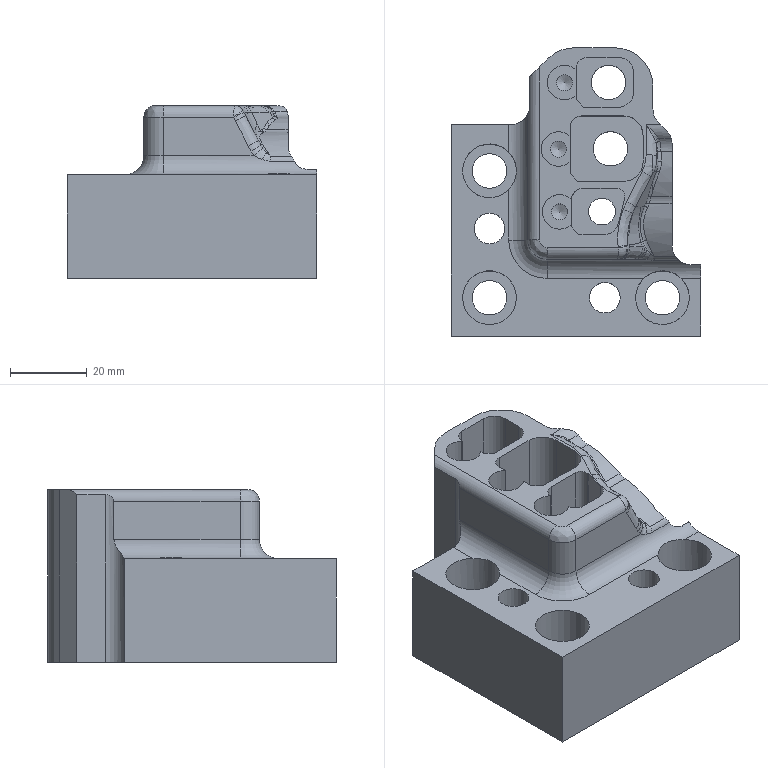Part | STEP file | 1 solid | 125 faces | box 65 x 75 x 45.001 mm | volume 106035 mm3 | cylinder 44 | plane 40 | spline 37 | cone 3 | torus 1 | commonest cylinder face diameters 10 x12 9 x8 6 x6 8 x6 4.2 x3 14 x3